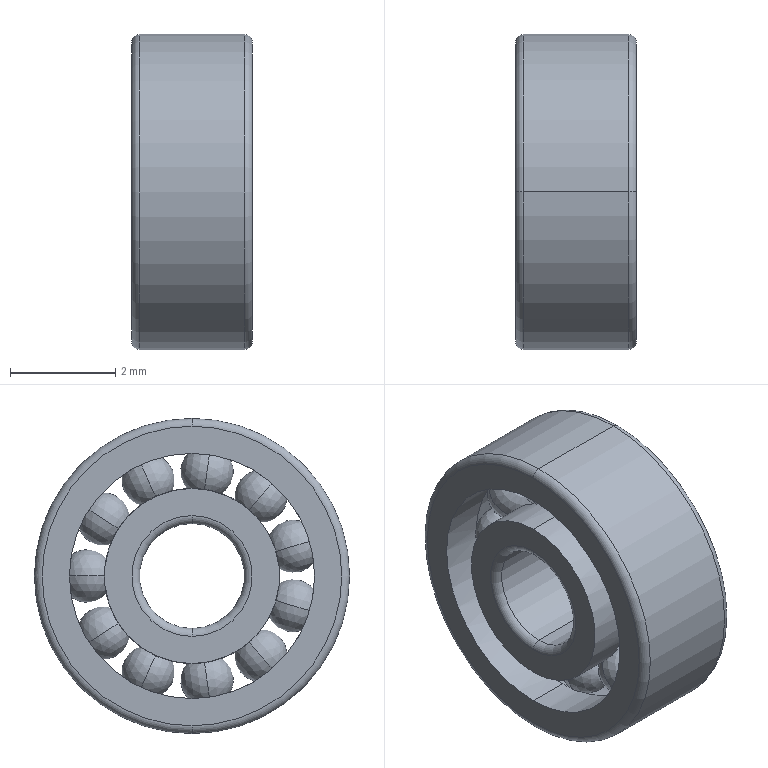Part | SolidWorks | features Stock 1 | 1 solid | 82 faces | box 2.3 x 6 x 6 mm | volume 42.074 mm3 | torus 44 | sphere 22 | cylinder 12 | plane 4 | commonest cylinder face diameters 3.333 x4 4.667 x4 2 x2 6 x2